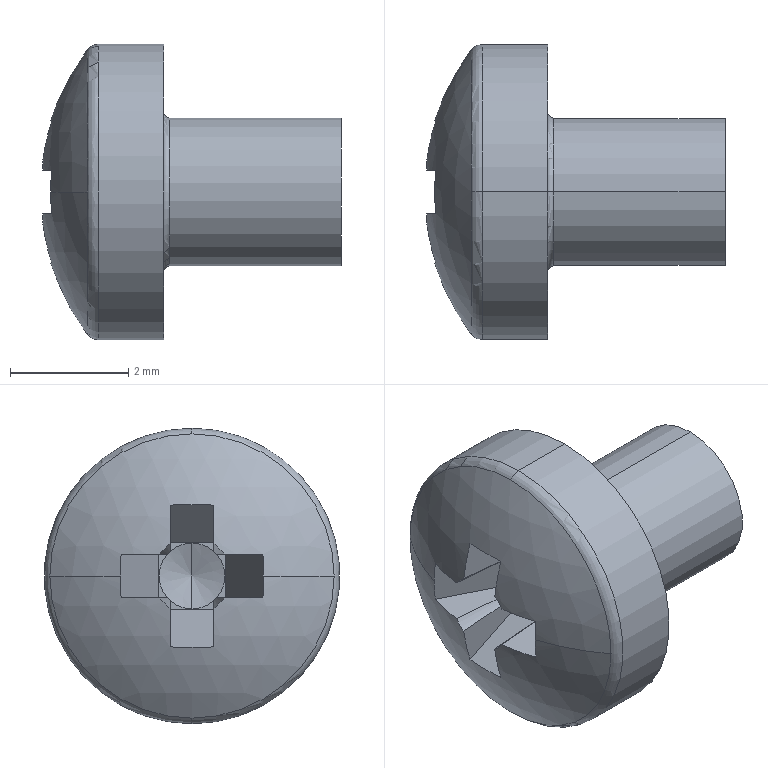Part | SolidWorks | features RevCut 2, BlendCut 1, CirPattern 1, Fillet 1, LPattern 1, Revolution 1 | 1 solid | 34 faces | box 5.046 x 5 x 5 mm | volume 44.537 mm3 | plane 18 | cone 6 | torus 4 | cylinder 4 | sphere 2 | commonest cylinder face diameters 2.5 x2 5 x2